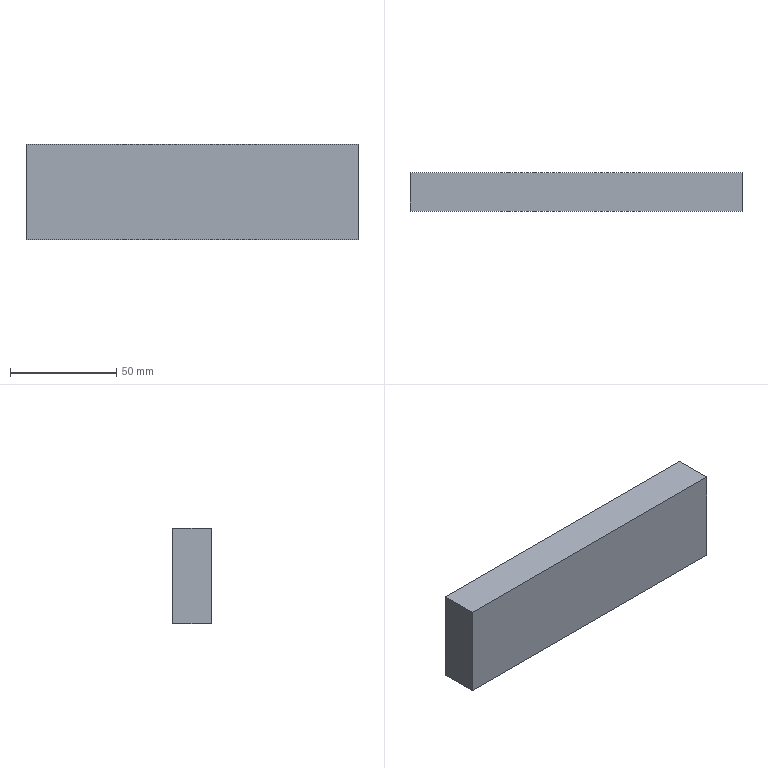NC program | NX | posted with a generic post | part box 156 x 18 x 45 mm
Lines 1 to 1294 of 3545:
N10 G17 G21 G94 G90
(PLANAR_MILL , TOOL : D16C)
N12 T01 M6
N14 G54
N16 G17 G0 G90 X-90. Y0. S2300 M3
N18 G43 Z20. H1
N20 Z3.
N22 G94 G1 Z0. F800.
N24 X-74.
N26 X74.
N28 X90.
N30 Z3.
N32 G0 Z20.
(ADAPTIVE_MILLING , TOOL : D16C)
N34 X93.024 Y6.776 S3500
N36 Z-38.
N38 G1 X92.875 Y6.789 Z-38.937 F1500.
N40 X92.725 Y6.801 Z-39.308
N42 X92.576 Y6.813 Z-39.58
N44 X92.426 Y6.826 Z-39.8
N46 X92.277 Y6.838 Z-39.984
N48 X92.127 Y6.85 Z-40.142
N50 X91.978 Y6.863 Z-40.28
N52 X91.828 Y6.875 Z-40.4
N54 X91.679 Y6.887 Z-40.505
N56 X91.529 Y6.9 Z-40.598
N58 X91.38 Y6.912 Z-40.679
N60 X91.231 Y6.924 Z-40.75
N62 X91.081 Y6.937 Z-40.81
N64 X90.932 Y6.949 Z-40.862
N66 X90.782 Y6.961 Z-40.905
N68 X90.633 Y6.974 Z-40.939
N70 X90.483 Y6.986 Z-40.966
N72 X90.334 Y6.998 Z-40.985
N74 X90.184 Y7.011 Z-40.996
N76 X90.035 Y7.023 Z-41.
N78 X87.714 Y7.215
N80 G3 X86.001 Y5.942 R1.616
N82 X85.745 Y2.219 R24.863
N84 X85.69 Y-7.255 R731.999
N86 G2 X82.243 Y-13.665 R8.873
N88 X76.479 Y-16.159 R12.982
N90 X70.319 Y-16.657 R37.349
N92 X60.044 Y-16.7 R710.459
N94 G1 X-75.926
N96 G2 X-82.503 Y-13.438 R8.777
N98 X-85.116 Y-7.695 R12.719
N100 X-85.653 Y-1.502 R35.427
N102 X-85.678 Y7.423 R259.053
N104 X-82.107 Y13.763 R8.94
N106 X-76.314 Y16.188 R13.167
N108 X-70.377 Y16.655 R37.978
N110 X-60.252 Y16.7 R702.362
N112 G1 X76.02 Y16.698
N114 G2 X82.504 Y13.429 R8.805
N116 X85.03 Y7.644 R11.914
N118 X85.396 Y1.962 R36.217
N120 X85.378 Y-5.456 R267.86
N122 X80.394 Y-13.694 R10.594
N124 X74.115 Y-15.922 R15.915
N126 X67.459 Y-16.36 R49.943
N128 X57.034 Y-16.399 R727.387
N130 G1 X-73.776
N132 G2 X-82.645 Y-11.469 R10.563
N134 X-84.903 Y-5.239 R15.759
N136 X-85.356 Y1.303 R47.673
N138 X-85.348 Y5.689 R58.15
N140 X-80.369 Y13.704 R10.603
N142 X-74.26 Y15.898 R15.81
N144 X-67.344 Y16.362 R49.309
N146 X-58.119 Y16.399 R683.552
N148 G1 X73.914 Y16.397
N150 G2 X82.791 Y11.121 R10.428
N152 X84.753 Y4.979 R15.923
N154 X85.085 Y-1.983 R59.735
N156 X84.675 Y-6.373 R15.473
N158 X78.65 Y-13.752 R11.862
N160 X72.18 Y-15.676 R18.719
N162 X65.032 Y-16.065 R63.475
N164 G1 X54.757 Y-16.099
N166 X-72.087 Y-16.097
N168 G2 X-82.601 Y-9.926 R11.776
N170 X-84.63 Y-3.518 R18.113
N172 X-85.016 Y4.076 R47.717
N174 X-79.074 Y13.505 R11.652
N176 X-72.582 Y15.618 R17.858
N178 X-65.101 Y16.064 R59.034
N180 G1 X-54.751 Y16.099
N182 X71.888
N184 G2 X79.569 Y13.489 R11.642
N186 X83.651 Y7.131 R13.214
N188 X84.661 Y0.626 R26.639
N190 X84.592 Y-3.941 R24.232
N192 X82.297 Y-9.622 R12.908
N194 G1 X81.593 Y-10.791
N196 G2 X79.789 Y-12.594 R9.495
N198 X76.093 Y-14.321 R13.778
N200 X68.797 Y-15.587 R29.634
N202 X59.125 Y-15.792 R167.5
N204 G1 X52.825 Y-15.799
N206 X-71.108 Y-15.792
N208 G2 X-78.673 Y-13.273 R13.032
N210 X-80.764 Y-11.762 R9.397
N212 X-82.832 Y-8.434 R9.597
N214 X-84.494 Y-0.994 R25.738
N216 X-84.56 Y3.722 R23.424
N218 X-82.359 Y9.479 R12.307
N220 X-81.593 Y10.791 R11.314
N222 X-79.789 Y12.594 R9.495
N224 X-76.126 Y14.308 R13.699
N226 X-68.905 Y15.579 R29.459
N228 X-59.459 Y15.791 R157.993
N230 G1 X-52.859 Y15.798
N232 X71.104 Y15.792
N234 G2 X78.874 Y13.025 R12.62
N236 G1 X79.791 Y12.463
N238 G2 X81.594 Y10.659 R9.495
N240 X82.435 Y9.194 R10.523
N242 X84.216 Y1.4 R25.74
N244 X83.999 Y-4.16 R18.18
N246 X83.097 Y-6.98 R20.614
N248 G1 X83.059 Y-7.164
N250 G3 X83.597 Y-8.552 R1.601
N252 X84.161 Y-8.878 Z-40.979 R1.942
N254 G1 X86.488 Y-9.882 Z-40.9
N256 X87.519 Y-10.327 F15000.
N258 G2 X86.647 Y-13.378 R1.6
N260 G1 X85.769 Y-13.25
N262 X84.762 Y-13.23
N264 X81.573 Y-13.177 Z-41. F1500.
N266 X79.337 Y-13.141
N268 G3 X78.699 Y-13.262 R1.629
N270 G1 X77.517 Y-13.751
N272 G2 X65.466 Y-15.396 R50.543
N274 X51.291 Y-15.498 R552.582
N276 G1 X-70.945 Y-15.497
N278 G2 X-76.206 Y-14.066 R17.016
N280 G1 X-77.52 Y-13.751
N282 X-78.697 Y-13.263
N284 G3 X-80.899 Y-14.551 R1.6
N286 X-80.499 Y-15.822 Z-40.957 R1.683
N288 G1 X-79.408 Y-17.277 Z-40.9
N290 X-78.351 Y-18.687 F15000.
N292 G3 X-77.072 Y-19.328 R1.601
N294 G1 X73.134 Y-19.488
N296 G3 X74.042 Y-19.206 R1.606
N298 G1 X75.642 Y-18.107
N300 X76.516 Y-17.511 Z-40.933 F1500.
N302 X77.382 Y-16.903 Z-40.966
N304 G3 X77.954 Y-16.021 Z-41. R1.6
N306 X76.274 Y-14.05 R1.6
N308 X71.939 Y-14.58 R95.722
N310 G2 X61.46 Y-15.159 R95.011
N312 X50.51 Y-15.198 R758.856
N314 G1 X-70.92 Y-15.197
N316 G2 X-74.563 Y-14.26 R24.752
N318 G1 X-75.033 Y-14.147
N320 G2 X-76.458 Y-14.006 R10.128
N322 G3 X-78.339 Y-16.099 R1.6
N324 X-77.575 Y-16.987 Z-40.963 R1.702
N326 G1 X-75.904 Y-18.072 Z-40.9
N328 X-74.189 Y-19.185 F15000.
N330 G3 X-73.319 Y-19.443 R1.608
N332 G1 X72.573 Y-19.532
N334 G3 X73.481 Y-19.25 R1.606
N336 G1 X75.095 Y-18.141
N338 X76.812 Y-16.956 Z-40.965 F1500.
N340 G3 X77.398 Y-16.048 Z-41. R1.601
N342 X75.713 Y-14.094 R1.6
N344 G2 X73.463 Y-14.201 R70.607
N346 X58.022 Y-14.88 R160.391
N348 G1 X48.722 Y-14.897
N350 X-68.72 Y-14.896
N352 G2 X-73.459 Y-14.172 R28.882
N354 G3 X-75.038 Y-14.147 R19.275
N356 X-76.744 Y-15.99 R1.6
N358 X-76.07 Y-17.061 Z-40.959 R1.617
N360 G1 X-74.513 Y-18.13 Z-40.9
N362 X-72.804 Y-19.304 F15000.
N364 G3 X-71.898 Y-19.585 R1.606
N366 G1 X71.372 Y-19.588
N368 G3 X72.301 Y-19.291 R1.605
N370 G1 X73.908 Y-18.146
N372 X74.713 Y-17.574 Z-40.931 F1500.
N374 X75.513 Y-16.994 Z-40.962
N376 G3 X76.097 Y-15.965 Z-41. R1.6
N378 X74.512 Y-14.15 R1.6
N380 X67.386 Y-14.354 R97.044
N382 G2 X52.801 Y-14.594 R328.555
N384 G1 X47.626 Y-14.597
N386 X-68.72 Y-14.596
N388 G2 X-71.854 Y-14.15 R102.479
N390 G1 X-73.692
N392 G3 X-75.281 Y-15.935 R1.6
N394 X-74.622 Y-17.051 Z-40.958 R1.617
N396 G1 X-73.114 Y-18.13 Z-40.9
N398 X-71.494 Y-19.289 F15000.
N400 G3 X-70.552 Y-19.588 R1.605
N402 G1 X67.597 Y-18.59
N404 X67.807 Y-18.573
N406 X68.015 Y-18.531
N408 X69.418 Y-18.14
N410 X72.49 Y-17.284 Z-41. F1500.
N412 G3 X72.037 Y-14.15 R1.6
N414 X58.515 Y-14.265 R663.31
N416 G1 X47.34 Y-14.297
N418 X-66.61 Y-14.293
N420 G2 X-68.97 Y-14.15 R55.681
N422 G1 X-71.857
N424 G3 X-72.343 Y-17.274 R1.6
N426 G1 X-69.272 Y-18.133 Z-40.9
N428 X-68.49 Y-18.354 F15000.
N430 X-67.706 Y-18.564
N432 X-67.417 Y-18.59
N434 X61.934
N436 X62.151 Y-18.573
N438 X62.365 Y-18.531
N440 X63.761 Y-18.141
N442 X66.833 Y-17.283 Z-41. F1500.
N444 G3 X66.374 Y-14.15 R1.6
N446 G1 X-75.001
N448 G2 X-77.52 Y-13.751 R9.498
N450 X-79.791 Y-12.593 R9.495
N452 X-81.594 Y-10.789 R9.495
N454 X-82.751 Y-8.517 R9.495
N456 X-84.2 Y0.015 R46.979
N458 X-83.114 Y6.806 R15.168
N460 G1 X-83.069 Y7.026
N462 G3 X-84.767 Y8.747 R1.6
N464 X-85.905 Y8.161 Z-40.959 R1.617
N466 G1 X-87.087 Y6.709 Z-40.9
N468 X-88.925 Y4.452 F15000.
N470 G3 X-89.284 Y3.438 R1.603
N472 G1 X-89.264 Y-3.686
N474 G3 X-88.906 Y-4.69 R1.604
N476 G1 X-87.084 Y-6.933
N478 X-85.825 Y-8.476 Z-40.962 F1500.
N480 G3 X-84.777 Y-8.994 Z-41. R1.6
N482 X-83.05 Y-7.274 R1.6
N484 X-83.574 Y-2.989 R93.564
N486 G2 X-83.595 Y2.99 R20.7
N488 G1 X-83.151 Y5.291
N490 G2 X-83.049 Y7.276 R15.825
N492 G1 X-82.751 Y8.52
N494 X-82.32 Y9.559
N496 G3 X-84.889 Y11.342 R1.6
N498 G1 X-85.092 Y11.113 Z-40.99
N500 X-85.272 Y10.865 Z-40.981
N502 X-86.783 Y8.779 Z-40.9
N504 X-88.236 Y6.774 F15000.
N506 G3 X-88.535 Y5.971 R1.61
N508 G1 X-89.309 Y-3.125
N510 G3 X-88.936 Y-4.294 R1.602
N512 G1 X-87.126 Y-6.434
N514 X-86.49 Y-7.19 Z-40.931 F1500.
N516 X-85.846 Y-7.939 Z-40.962
N518 G3 X-84.773 Y-8.436 Z-41. R1.6
N520 X-83.094 Y-6.713 R1.6
N522 G2 X-83.202 Y-4.439 R74.089
N524 X-83.395 Y0.423 R39.504
N526 X-83.15 Y2.998 R43.005
N528 G1 Y5.332
N530 G3 X-85.913 Y6.431 R1.6
N532 X-86.306 Y5.737 Z-40.975 R1.812
N534 G1 X-87.133 Y3.499 Z-40.9
N536 X-88.125 Y0.812 F15000.
N538 G3 X-88.224 Y0.258 R1.667
N540 G1 X-88.226 Y-0.184
N542 X-88.213 Y-0.626
N544 X-88.178 Y-0.811
N546 X-88.125 Y-0.992
N548 X-87.141 Y-3.655
N550 X-86.251 Y-6.066 Z-40.981 F1500.
N552 G3 X-85.931 Y-6.592 Z-41. R1.636
N554 X-83.15 Y-5.512 R1.6
N556 G1 Y6.001
N558 G2 X-82.751 Y8.52 R9.498
N560 X-81.593 Y10.791 R9.495
N562 X-79.789 Y12.594 R9.495
N564 X-77.517 Y13.751 R9.495
N566 X-65.692 Y15.388 R50.154
N568 X-51.293 Y15.498 R516.951
N570 G1 X70.907 Y15.497
N572 G2 X76.456 Y13.882 R16.043
N574 X78.893 Y13.013 R8.415
N576 G3 X81.329 Y14.401 R1.6
N578 X80.886 Y15.493 Z-40.962 R1.701
N580 G1 X79.651 Y17.047 Z-40.9
N582 X78.516 Y18.474 F15000.
N584 G3 X77.268 Y19.079 R1.601
N586 G1 X-73.134 Y19.488
N588 G3 X-74.045 Y19.206 R1.606
N590 G1 X-75.643 Y18.107
N592 X-76.517 Y17.511 Z-40.933 F1500.
N594 X-77.383 Y16.903 Z-40.966
N596 G3 X-77.955 Y16.019 Z-41. R1.6
N598 X-76.274 Y14.05 R1.6
N600 X-71.912 Y14.583 R96.343
N602 G2 X-61.433 Y15.159 R95.363
N604 X-50.334 Y15.198 R764.363
N606 G1 X70.891 Y15.197
N608 G2 X74.679 Y14.163 R21.713
N610 G3 X75.293 Y13.997 R10.655
N612 G2 X76.531 Y13.858 R6.686
N614 G3 X78.403 Y15.976 R1.6
N616 X77.646 Y16.84 Z-40.963 R1.707
N618 G1 X75.955 Y17.938 Z-40.9
N620 X74.26 Y19.038 F15000.
N622 G3 X73.392 Y19.296 R1.608
N624 G1 X-72.573 Y19.532
N626 G3 X-73.482 Y19.25 R1.606
N628 G1 X-75.096 Y18.141
N630 X-76.812 Y16.956 Z-40.965 F1500.
N632 G3 X-77.398 Y16.047 Z-41. R1.601
N634 X-75.713 Y14.094 R1.6
N636 G2 X-73.44 Y14.202 R73.267
N638 X-57.996 Y14.88 R160.551
N640 G1 X-48.696 Y14.897
N642 X70.328 Y14.898
N644 G2 X72.74 Y14.355 R16.77
N646 G3 X74.167 Y14.02 R11.704
N648 G2 X75.3 Y13.996 R29.277
N650 G3 X77. Y15.876 R1.6
N652 X76.209 Y16.994 Z-40.956 R1.677
N654 G1 X74.744 Y18. Z-40.9
N656 X73.064 Y19.153 F15000.
N658 G3 X72.16 Y19.434 R1.606
N660 G1 X-71.372 Y19.588
N662 G3 X-72.303 Y19.291 R1.605
N664 G1 X-73.908 Y18.146
N666 X-74.714 Y17.574 Z-40.931 F1500.
N668 X-75.514 Y16.994 Z-40.962
N670 G3 X-76.097 Y15.964 Z-41. R1.6
N672 X-74.512 Y14.15 R1.6
N674 X-67.173 Y14.364 R103.503
N676 G2 X-52.851 Y14.593 R332.279
N678 G1 X-47.601 Y14.597
N680 X69.293
N682 G2 X72.647 Y14.021 R67.717
N684 G1 X74.184 Y14.02
N686 G3 X75.773 Y15.805 R1.6
N688 X75.115 Y16.921 Z-40.958 R1.617
N690 G1 X73.606 Y18. Z-40.9
N692 X71.985 Y19.159 F15000.
N694 G3 X71.045 Y19.458 R1.605
N696 G1 X-67.634 Y18.59
N698 X-67.846 Y18.573
N700 X-68.054 Y18.531
N702 X-69.457 Y18.14
N704 X-72.529 Y17.284 Z-41. F1500.
N706 G3 X-72.074 Y14.15 R1.6
N708 X-58.452 Y14.266 R673.335
N710 G1 X-47.127 Y14.297
N712 X68.408 Y14.296
N714 X70.609 Y14.02
N716 X72.709
N718 G3 X74.298 Y15.805 R1.6
N720 X73.64 Y16.921 Z-40.958 R1.617
N722 G1 X72.131 Y18. Z-40.9
N724 X70.511 Y19.159 F15000.
N726 G3 X69.569 Y19.458 R1.605
N728 G1 X-61.934 Y18.59
N730 X-62.146 Y18.573
N732 X-62.353 Y18.531
N734 X-63.756 Y18.14
N736 X-66.829 Y17.284 Z-41. F1500.
N738 G3 X-66.374 Y14.15 R1.6
N740 G1 X54.5
N742 G3 X60.001 Y14.02 R82.862
N744 G1 X70.613
N746 G3 X71.704 Y16.79 R1.6
N748 X71.024 Y17.174 Z-40.975 R1.783
N750 G1 X68.769 Y18.003 Z-40.9
N752 X66.067 Y18.996 F15000.
N754 G3 X65.539 Y19.094 R1.682
N756 G1 X60.436 Y19.171
N758 G3 X59.844 Y19.068 R1.64
N760 G1 X56.792 Y17.91
N762 X55.796 Y17.536 Z-40.933 F1500.
N764 X54.804 Y17.151 Z-40.967
N766 G3 X54.044 Y16.439 Z-41. R1.6
N768 X55.361 Y14.097 R1.6
N770 X58.272 Y13.823 R18.352
N772 G1 X58.383 Y13.839
N774 G3 X58.195 Y17.312 R1.76
N776 G1 X56.437 Y17.488
N778 G3 X55.94 Y14.006 R1.76
N780 X57.744 Y13.716 R12.424
N782 X58.7 Y13.916 R6.013
N784 G1 X59.896 Y14.012
N786 G3 X59.639 Y17.522 R1.76
N788 G1 X56.894 Y17.34
N790 G3 X56.48 Y13.906 R1.76
N792 X57.713 Y13.684 R2.819
N794 G1 X58.018 Y13.748
N796 G3 X57.273 Y17.187 R1.76
N798 X55.768 Y15.843 R1.792
N800 X56.945 Y13.759 R1.76
N802 X58.229 Y13.796 R2.153
N804 G1 X58.7 Y13.916
N806 X60.001 Y14.02
N808 X75.001
N810 G2 X77.52 Y13.621 R9.498
N812 X79.791 Y12.463 R9.495
N814 X81.594 Y10.659 R9.495
N816 X82.751 Y8.387 R9.495
N818 X83.606 Y3.684 R39.624
N820 X83.803 Y-2.072 R23.31
N822 X83.158 Y-5.447 R35.619
N824 X83.049 Y-7.276 R22.868
N826 X82.277 Y-9.663 R9.423
N828 G3 X84.875 Y-11.418 R1.6
N830 G1 X85.062 Y-11.199 Z-40.991
N832 X85.231 Y-10.966 Z-40.982
N834 X86.766 Y-8.851 Z-40.9
N836 X88.192 Y-6.887 F15000.
N838 G3 X88.492 Y-6.075 R1.609
N840 G1 X89.264 Y3.556
N842 G3 X88.893 Y4.715 R1.602
N844 G1 X87.083 Y6.861
N846 X86.447 Y7.618 Z-40.931 F1500.
N848 X85.804 Y8.369 Z-40.962
N850 G3 X84.731 Y8.867 Z-41. R1.6
N852 X83.05 Y7.144 R1.6
N854 G2 X83.492 Y1.524 R292.083
N856 X83.15 Y-3.478 R26.196
N858 G1 Y-5.578
N860 G3 X84.75 Y-7.178 R1.6
N862 X85.975 Y-6.607 Z-40.956 R1.612
N864 G1 X87.129 Y-5.233 Z-40.9
N866 X88.99 Y-3.019 F15000.
N868 G3 X89.365 Y-1.989 R1.603
N870 G1 Y2.281
N872 G3 X88.99 Y3.311 R1.603
N874 G1 X87.148 Y5.503
N876 X86.533 Y6.24 Z-40.93 F1500.
N878 X85.908 Y6.969 Z-40.96
N880 G3 X84.779 Y7.469 Z-41. R1.599
N882 X83.15 Y5.869 R1.6
N884 G2 X83.15 Y-3.503 R737.034
N886 G3 X84.75 Y-5.103 R1.6
N888 X85.975 Y-4.532 Z-40.956 R1.612
N890 G1 X87.129 Y-3.159 Z-40.9
N892 X88.99 Y-0.944 F15000.
N894 G3 X89.365 Y0.085 R1.603
N896 X89.322 Y0.738 R2.708
N898 X88.99 Y1.398 R1.617
N900 G1 X87.148 Y3.591
N902 X86.533 Y4.328 Z-40.93 F1500.
N904 X85.908 Y5.057 Z-40.96
N906 G3 X84.779 Y5.557 Z-41. R1.599
N908 X83.15 Y3.957 R1.6
N910 G1 Y0.469
N912 G3 X84.543 Y-1.131 R1.616
N914 G1 X87.137 Y-1.492
N916 X87.285 Y-1.513 Z-40.996
N918 X87.434 Y-1.534 Z-40.985
N920 X87.582 Y-1.554 Z-40.966
N922 X87.731 Y-1.575 Z-40.939
N924 X87.88 Y-1.596 Z-40.905
N926 X88.028 Y-1.617 Z-40.862
N928 X88.177 Y-1.637 Z-40.81
N930 X88.325 Y-1.658 Z-40.75
N932 X88.474 Y-1.679 Z-40.679
N934 X88.622 Y-1.699 Z-40.598
N936 X88.771 Y-1.72 Z-40.505
N938 X88.92 Y-1.741 Z-40.4
N940 X89.068 Y-1.761 Z-40.28
N942 X89.217 Y-1.782 Z-40.142
N944 X89.365 Y-1.803 Z-39.984
N946 X89.514 Y-1.823 Z-39.8
N948 X89.662 Y-1.844 Z-39.58
N950 X89.811 Y-1.865 Z-39.308
N952 X89.959 Y-1.886 Z-38.937
N954 X90.108 Y-1.906 Z-38.
N956 G0 Z20.
N958 M5
(PLANAR_MILL_1 , TOOL : D14J)
N960 T02 M6
N962 G54
N964 G17 G0 G90 X55.513 Y15.492 S3000 M3
N966 G43 Z20. H2
N968 Z-39.
N970 G94 G1 Z-41. F600.
N972 G41 X55.426 Y15. D2
N974 G3 X57.426 Y13. R2.
N976 G1 X75.
N978 G2 X82. Y6. R7.
N980 G1 Y-6.
N982 G2 X75. Y-13. R7.
N984 G1 X-75.
N986 G2 X-82. Y-6. R7.
N988 G1 Y6.
N990 G2 X-75. Y13. R7.
N992 G1 X57.426
N994 G3 X59.426 Y15. R2.
N996 G40
N998 G1 X59.339 Y15.492
N1000 X55.513
N1002 G41 X55.426 Y15.
N1004 G3 X57.426 Y13. R2.
N1006 G1 X75.
N1008 G2 X82. Y6. R7.
N1010 G1 Y-6.
N1012 G2 X75. Y-13. R7.
N1014 G1 X-75.
N1016 G2 X-82. Y-6. R7.
N1018 G1 Y6.
N1020 G2 X-75. Y13. R7.
N1022 G1 X57.426
N1024 G3 X59.426 Y15. R2.
N1026 G40
N1028 G1 X59.339 Y15.492
N1030 Z-39.
N1032 G0 Z20.
(PLANAR_MILL_1_COPY_1 , TOOL : D14J)
N1034 X57.087 Y15.362
N1036 Z-39.
N1038 G1 Z-41.
N1040 G41 X57. Y14.87
N1042 G3 X59. Y12.87 R2.
N1044 G1 X75.5
N1046 G3 X77.5 Y14.87 R2.
N1048 G40
N1050 G1 X77.413 Y15.362
N1052 Z-39.
N1054 G0 Z20.
N1056 X57.087
N1058 Z-39.
N1060 G1 Z-41.
N1062 G41 X57. Y14.87
N1064 G3 X59. Y12.87 R2.
N1066 G1 X75.5
N1068 G3 X77.5 Y14.87 R2.
N1070 G40
N1072 G1 X77.413 Y15.362
N1074 Z-39.
N1076 G0 Z20.
N1078 M5
(PLANAR_MILL_2 , TOOL : D4C)
N1080 T03 M6
N1082 G54
N1084 G17 G0 G90 X-5.194 Y1.15 S3500 M3
N1086 G43 Z20. H3
N1088 Z0.5
N1090 G94 G1 X-69.264 Z0.444 F1500.
N1092 X-69.834 Y0.834
N1094 X-70.15 Y0.264 Z0.443
N1096 Y-0.264 Z0.442
N1098 X-69.834 Y-0.834
N1100 X-69.264 Y-1.15 Z0.441
N1102 X46.264 Z0.341
N1104 G3 X46.958 Y0.689 R1.222
N1106 G1 X46.653 Y0.983 Z0.338
N1108 X46.264 Y1.15
N1110 X-69.264 Z0.237
N1112 X-69.834 Y0.834 Z0.236
N1114 X-70.15 Y0.264
N1116 Y-0.264 Z0.235
N1118 X-69.834 Y-0.834
N1120 X-69.264 Y-1.15 Z0.234
N1122 X46.264 Z0.133
N1124 G3 X46.958 Y0.689 R1.222
N1126 G1 X46.653 Y0.983 Z0.131
N1128 X46.264 Y1.15
N1130 X-69.264 Z0.03
N1132 X-69.834 Y0.834 Z0.029
N1134 X-70.15 Y0.264
N1136 Y-0.264 Z0.028
N1138 X-69.834 Y-0.834
N1140 X-69.264 Y-1.15 Z0.027
N1142 X46.264 Z-0.074
N1144 G3 X46.958 Y0.689 R1.222
N1146 G1 X46.653 Y0.983 Z-0.076
N1148 X46.264 Y1.15
N1150 X-69.264 Z-0.177
N1152 X-69.834 Y0.834 Z-0.178
N1154 X-70.15 Y0.264
N1156 Y-0.264 Z-0.179
N1158 X-69.834 Y-0.834
N1160 X-69.264 Y-1.15 Z-0.18
N1162 X46.264 Z-0.281
N1164 G3 X46.958 Y0.689 R1.222
N1166 G1 X46.653 Y0.983 Z-0.283
N1168 X46.264 Y1.15 Z-0.284
N1170 X-69.264 Z-0.384
N1172 X-69.834 Y0.834 Z-0.385
N1174 X-70.15 Y0.264
N1176 Y-0.264 Z-0.386
N1178 X-69.834 Y-0.834 Z-0.387
N1180 X-69.264 Y-1.15
N1182 X46.264 Z-0.488
N1184 G3 X46.958 Y0.689 R1.222
N1186 G1 X46.653 Y0.983 Z-0.49
N1188 X46.264 Y1.15 Z-0.491
N1190 X-69.264 Z-0.591
N1192 X-69.834 Y0.834 Z-0.592
N1194 X-70.15 Y0.264 Z-0.593
N1196 Y-0.264
N1198 X-69.834 Y-0.834 Z-0.594
N1200 X-69.264 Y-1.15
N1202 X46.264 Z-0.695
N1204 G3 X46.958 Y0.689 R1.222
N1206 G1 X46.653 Y0.983 Z-0.697
N1208 X46.264 Y1.15 Z-0.698
N1210 X-69.264 Z-0.799
N1212 X-69.834 Y0.834
N1214 X-70.15 Y0.264 Z-0.8
N1216 Y-0.264
N1218 X-69.834 Y-0.834 Z-0.801
N1220 X-69.264 Y-1.15
N1222 X46.264 Z-0.902
N1224 G3 X46.958 Y0.689 R1.222
N1226 G1 X46.653 Y0.983 Z-0.904
N1228 X46.264 Y1.15 Z-0.905
N1230 X-69.264 Z-1.006
N1232 X-69.834 Y0.834
N1234 X-70.15 Y0.264 Z-1.007
N1236 Y-0.264
N1238 X-69.834 Y-0.834 Z-1.008
N1240 X-69.264 Y-1.15
N1242 X46.264 Z-1.109
N1244 G3 X46.958 Y0.689 R1.222
N1246 G1 X46.653 Y0.983 Z-1.112
N1248 X46.264 Y1.15
N1250 X-69.264 Z-1.213
N1252 X-69.834 Y0.834
N1254 X-70.15 Y0.264 Z-1.214
N1256 Y-0.264
N1258 X-69.834 Y-0.834 Z-1.215
N1260 X-69.264 Y-1.15 Z-1.216
N1262 X46.264 Z-1.316
N1264 G3 X46.958 Y0.689 R1.222
N1266 G1 X46.653 Y0.983 Z-1.319
N1268 X46.264 Y1.15
N1270 X-69.264 Z-1.42
N1272 X-69.834 Y0.834
N1274 X-70.15 Y0.264 Z-1.421
N1276 Y-0.264
N1278 X-69.834 Y-0.834 Z-1.422
N1280 X-69.264 Y-1.15 Z-1.423
N1282 X46.264 Z-1.523
N1284 G3 X46.958 Y0.689 R1.222
N1286 G1 X46.653 Y0.983 Z-1.526
N1288 X46.264 Y1.15
N1290 X-69.264 Z-1.627
N1292 X-69.834 Y0.834 Z-1.628
N1294 X-70.15 Y0.264
N1296 Y-0.264 Z-1.629
N1298 X-69.834 Y-0.834
N1300 X-69.264 Y-1.15 Z-1.63
N1302 X46.264 Z-1.731
N1304 G3 X46.958 Y0.689 R1.222
N1306 G1 X46.653 Y0.983 Z-1.733
N1308 X46.264 Y1.15
N1310 X-69.264 Z-1.834
N1312 X-69.834 Y0.834 Z-1.835
N1314 X-70.15 Y0.264
N1316 Y-0.264 Z-1.836
N1318 X-69.834 Y-0.834
N1320 X-69.264 Y-1.15 Z-1.837
N1322 X46.264 Z-1.938
N1324 G3 X46.958 Y0.689 R1.222
N1326 G1 X46.653 Y0.983 Z-1.94
N1328 X46.264 Y1.15
N1330 X-69.264 Z-2.041
N1332 X-69.834 Y0.834 Z-2.042
N1334 X-70.15 Y0.264
N1336 Y-0.264 Z-2.043
N1338 X-69.834 Y-0.834
N1340 X-69.264 Y-1.15 Z-2.044
N1342 X46.264 Z-2.145
N1344 G3 X46.958 Y0.689 R1.222
N1346 G1 X46.653 Y0.983 Z-2.147
N1348 X46.264 Y1.15 Z-2.148
N1350 X-69.264 Z-2.248
N1352 X-69.834 Y0.834 Z-2.249
N1354 X-70.15 Y0.264
N1356 Y-0.264 Z-2.25
N1358 X-69.834 Y-0.834
N1360 X-69.264 Y-1.15 Z-2.251
N1362 X46.264 Z-2.352
N1364 G3 X46.958 Y0.689 R1.222
N1366 G1 X46.653 Y0.983 Z-2.354
N1368 X46.264 Y1.15 Z-2.355
N1370 X-69.264 Z-2.455
N1372 X-69.834 Y0.834 Z-2.456
N1374 X-70.15 Y0.264 Z-2.457
N1376 Y-0.264
N1378 X-69.834 Y-0.834 Z-2.458
N1380 X-69.264 Y-1.15
N1382 X46.264 Z-2.559
N1384 G3 X46.958 Y0.689 R1.222
N1386 G1 X46.653 Y0.983 Z-2.561
N1388 X46.264 Y1.15 Z-2.562
N1390 X-69.264 Z-2.663
N1392 X-69.834 Y0.834
N1394 X-70.15 Y0.264 Z-2.664
N1396 Y-0.264
N1398 X-69.834 Y-0.834 Z-2.665
N1400 X-69.264 Y-1.15
N1402 X46.264 Z-2.766
N1404 G3 X46.958 Y0.689 R1.222
N1406 G1 X46.653 Y0.983 Z-2.768
N1408 X46.264 Y1.15 Z-2.769
N1410 X-69.264 Z-2.87
N1412 X-69.834 Y0.834
N1414 X-70.15 Y0.264 Z-2.871
N1416 Y-0.264
N1418 X-69.834 Y-0.834 Z-2.872
N1420 X-69.264 Y-1.15
N1422 X46.264 Z-2.973
N1424 G3 X46.958 Y0.689 R1.222
N1426 G1 X46.653 Y0.983 Z-2.976
N1428 X46.264 Y1.15
N1430 X-69.264 Z-3.077
N1432 X-69.834 Y0.834
N1434 X-70.15 Y0.264 Z-3.078
N1436 Y-0.264
N1438 X-69.834 Y-0.834 Z-3.079
N1440 X-69.264 Y-1.15
N1442 X46.264 Z-3.18
N1444 G3 X46.958 Y0.689 R1.222
N1446 G1 X46.653 Y0.983 Z-3.183
N1448 X46.264 Y1.15
N1450 X-69.264 Z-3.284
N1452 X-69.834 Y0.834
N1454 X-70.15 Y0.264 Z-3.285
N1456 Y-0.264
N1458 X-69.834 Y-0.834 Z-3.286
N1460 X-69.264 Y-1.15 Z-3.287
N1462 X46.264 Z-3.387
N1464 G3 X46.958 Y0.689 R1.222
N1466 G1 X46.653 Y0.983 Z-3.39
N1468 X46.264 Y1.15
N1470 X-69.264 Z-3.491
N1472 X-69.834 Y0.834 Z-3.492
N1474 X-70.15 Y0.264
N1476 Y-0.264 Z-3.493
N1478 X-69.834 Y-0.834
N1480 X-69.264 Y-1.15 Z-3.494
N1482 X46.264 Z-3.595
N1484 G3 X46.958 Y0.689 R1.222
N1486 G1 X46.653 Y0.983 Z-3.597
N1488 X46.264 Y1.15
N1490 X-69.264 Z-3.698
N1492 X-69.834 Y0.834 Z-3.699
N1494 X-70.15 Y0.264
N1496 Y-0.264 Z-3.7
N1498 X-69.834 Y-0.834
N1500 X-69.264 Y-1.15 Z-3.701
N1502 X46.264 Z-3.802
N1504 G3 X46.958 Y0.689 R1.222
N1506 G1 X46.653 Y0.983 Z-3.804
N1508 X46.264 Y1.15
N1510 X-69.264 Z-3.905
N1512 X-69.834 Y0.834 Z-3.906
N1514 X-70.15 Y0.264
N1516 Y-0.264 Z-3.907
N1518 X-69.834 Y-0.834
N1520 X-69.264 Y-1.15 Z-3.908
N1522 X46.264 Z-4.009
N1524 G3 X46.958 Y0.689 R1.222
N1526 G1 X46.653 Y0.983 Z-4.011
N1528 X46.264 Y1.15
N1530 X-69.264 Z-4.112
N1532 X-69.834 Y0.834 Z-4.113
N1534 X-70.15 Y0.264
N1536 Y-0.264 Z-4.114
N1538 X-69.834 Y-0.834
N1540 X-69.264 Y-1.15 Z-4.115
N1542 X46.264 Z-4.216
N1544 G3 X46.958 Y0.689 R1.222
N1546 G1 X46.653 Y0.983 Z-4.218
N1548 X46.264 Y1.15 Z-4.219
N1550 X-69.264 Z-4.319
N1552 X-69.834 Y0.834 Z-4.32
N1554 X-70.15 Y0.264 Z-4.321
N1556 Y-0.264
N1558 X-69.834 Y-0.834 Z-4.322
N1560 X-69.264 Y-1.15
N1562 X46.264 Z-4.423
N1564 G3 X46.958 Y0.689 R1.222
N1566 G1 X46.653 Y0.983 Z-4.425
N1568 X46.264 Y1.15 Z-4.426
N1570 X-69.264 Z-4.527
N1572 X-69.834 Y0.834
N1574 X-70.15 Y0.264 Z-4.528
N1576 Y-0.264
N1578 X-69.834 Y-0.834 Z-4.529
N1580 X-69.264 Y-1.15
N1582 X46.264 Z-4.63
N1584 G3 X46.958 Y0.689 R1.222
N1586 G1 X46.653 Y0.983 Z-4.632
N1588 X46.264 Y1.15 Z-4.633
N1590 X-69.264 Z-4.734
N1592 X-69.834 Y0.834
N1594 X-70.15 Y0.264 Z-4.735
N1596 Y-0.264
N1598 X-69.834 Y-0.834 Z-4.736
N1600 X-69.264 Y-1.15
N1602 X46.264 Z-4.837
N1604 G3 X46.958 Y0.689 R1.222
N1606 G1 X46.653 Y0.983 Z-4.84
N1608 X46.264 Y1.15
N1610 X-69.264 Z-4.941
N1612 X-69.834 Y0.834
N1614 X-70.15 Y0.264 Z-4.942
N1616 Y-0.264
N1618 X-69.834 Y-0.834 Z-4.943
N1620 X-69.264 Y-1.15
N1622 X46.264 Z-5.044
N1624 G3 X46.958 Y0.689 R1.222
N1626 G1 X46.653 Y0.983 Z-5.047
N1628 X46.264 Y1.15
N1630 X-69.264 Z-5.148
N1632 X-69.834 Y0.834
N1634 X-70.15 Y0.264 Z-5.149
N1636 Y-0.264
N1638 X-69.834 Y-0.834 Z-5.15
N1640 X-69.264 Y-1.15 Z-5.151
N1642 X46.264 Z-5.251
N1644 G3 X46.958 Y0.689 R1.222
N1646 G1 X46.653 Y0.983 Z-5.254
N1648 X46.264 Y1.15
N1650 X-69.264 Z-5.355
N1652 X-69.834 Y0.834 Z-5.356
N1654 X-70.15 Y0.264
N1656 Y-0.264 Z-5.357
N1658 X-69.834 Y-0.834
N1660 X-69.264 Y-1.15 Z-5.358
N1662 X46.264 Z-5.458
N1664 G3 X46.958 Y0.689 R1.222
N1666 G1 X46.653 Y0.983 Z-5.461
N1668 X46.264 Y1.15
N1670 X-69.264 Z-5.562
N1672 X-69.834 Y0.834 Z-5.563
N1674 X-70.15 Y0.264
N1676 Y-0.264 Z-5.564
N1678 X-69.834 Y-0.834
N1680 X-69.264 Y-1.15 Z-5.565
N1682 X46.264 Z-5.666
N1684 G3 X46.958 Y0.689 R1.222
N1686 G1 X46.653 Y0.983 Z-5.668
N1688 X46.264 Y1.15
N1690 X-69.264 Z-5.769
N1692 X-69.834 Y0.834 Z-5.77
N1694 X-70.15 Y0.264
N1696 Y-0.264 Z-5.771
N1698 X-69.834 Y-0.834
N1700 X-69.264 Y-1.15 Z-5.772
N1702 X46.264 Z-5.873
N1704 G3 X46.958 Y0.689 R1.222
N1706 G1 X46.653 Y0.983 Z-5.875
N1708 X46.264 Y1.15
N1710 X-69.264 Z-5.976
N1712 X-69.834 Y0.834 Z-5.977
N1714 X-70.15 Y0.264
N1716 Y-0.264 Z-5.978
N1718 X-69.834 Y-0.834
N1720 X-69.264 Y-1.15 Z-5.979
N1722 X46.264 Z-6.08
N1724 G3 X46.958 Y0.689 R1.222
N1726 G1 X46.653 Y0.983 Z-6.082
N1728 X46.264 Y1.15 Z-6.083
N1730 X-69.264 Z-6.183
N1732 X-69.834 Y0.834 Z-6.184
N1734 X-70.15 Y0.264 Z-6.185
N1736 Y-0.264
N1738 X-69.834 Y-0.834 Z-6.186
N1740 X-69.264 Y-1.15
N1742 X46.264 Z-6.287
N1744 G3 X46.958 Y0.689 R1.222
N1746 G1 X46.653 Y0.983 Z-6.289
N1748 X46.264 Y1.15 Z-6.29
N1750 X-69.264 Z-6.39
N1752 X-69.834 Y0.834 Z-6.391
N1754 X-70.15 Y0.264 Z-6.392
N1756 Y-0.264
N1758 X-69.834 Y-0.834 Z-6.393
N1760 X-69.264 Y-1.15
N1762 X46.264 Z-6.494
N1764 G3 X46.958 Y0.689 R1.222
N1766 G1 X46.653 Y0.983 Z-6.496
N1768 X46.264 Y1.15 Z-6.497
N1770 X-69.264 Z-6.598
N1772 X-69.834 Y0.834
N1774 X-70.15 Y0.264 Z-6.599
N1776 Y-0.264
N1778 X-69.834 Y-0.834 Z-6.6
N1780 X-69.264 Y-1.15
N1782 X46.264 Z-6.701
N1784 G3 X46.958 Y0.689 R1.222
N1786 G1 X46.653 Y0.983 Z-6.704
N1788 X46.264 Y1.15
N1790 X-69.264 Z-6.805
N1792 X-69.834 Y0.834
N1794 X-70.15 Y0.264 Z-6.806
N1796 Y-0.264
N1798 X-69.834 Y-0.834 Z-6.807
N1800 X-69.264 Y-1.15
N1802 X46.264 Z-6.908
N1804 G3 X46.958 Y0.689 R1.222
N1806 G1 X46.653 Y0.983 Z-6.911
N1808 X46.264 Y1.15
N1810 X-69.264 Z-7.012
N1812 X-69.834 Y0.834
N1814 X-70.15 Y0.264 Z-7.013
N1816 Y-0.264
N1818 X-69.834 Y-0.834 Z-7.014
N1820 X-69.264 Y-1.15 Z-7.015
N1822 X46.264 Z-7.115
N1824 G3 X46.958 Y0.689 R1.222
N1826 G1 X46.653 Y0.983 Z-7.118
N1828 X46.264 Y1.15
N1830 X-69.264 Z-7.219
N1832 X-69.834 Y0.834
N1834 X-70.15 Y0.264 Z-7.22
N1836 Y-0.264 Z-7.221
N1838 X-69.834 Y-0.834
N1840 X-69.264 Y-1.15 Z-7.222
N1842 X46.264 Z-7.322
N1844 G3 X46.958 Y0.689 R1.222
N1846 G1 X46.653 Y0.983 Z-7.325
N1848 X46.264 Y1.15
N1850 X-69.264 Z-7.426
N1852 X-69.834 Y0.834 Z-7.427
N1854 X-70.15 Y0.264
N1856 Y-0.264 Z-7.428
N1858 X-69.834 Y-0.834
N1860 X-69.264 Y-1.15 Z-7.429
N1862 X46.264 Z-7.53
N1864 G3 X46.958 Y0.689 R1.222
N1866 G1 X46.653 Y0.983 Z-7.532
N1868 X46.264 Y1.15
N1870 X-69.264 Z-7.633
N1872 X-69.834 Y0.834 Z-7.634
N1874 X-70.15 Y0.264
N1876 Y-0.264 Z-7.635
N1878 X-69.834 Y-0.834
N1880 X-69.264 Y-1.15 Z-7.636
N1882 X46.264 Z-7.737
N1884 G3 X46.958 Y0.689 R1.222
N1886 G1 X46.653 Y0.983 Z-7.739
N1888 X46.264 Y1.15
N1890 X-69.264 Z-7.84
N1892 X-69.834 Y0.834 Z-7.841
N1894 X-70.15 Y0.264
N1896 Y-0.264 Z-7.842
N1898 X-69.834 Y-0.834
N1900 X-69.264 Y-1.15 Z-7.843
N1902 X46.264 Z-7.944
N1904 G3 X46.958 Y0.689 R1.222
N1906 G1 X46.653 Y0.983 Z-7.946
N1908 X46.264 Y1.15 Z-7.947
N1910 X-69.264 Z-8.047
N1912 X-69.834 Y0.834 Z-8.048
N1914 X-70.15 Y0.264
N1916 Y-0.264 Z-8.049
N1918 X-69.834 Y-0.834 Z-8.05
N1920 X-69.264 Y-1.15
N1922 X46.264 Z-8.151
N1924 G3 X46.958 Y0.689 R1.222
N1926 G1 X46.653 Y0.983 Z-8.153
N1928 X46.264 Y1.15 Z-8.154
N1930 X-69.264 Z-8.254
N1932 X-69.834 Y0.834 Z-8.255
N1934 X-70.15 Y0.264 Z-8.256
N1936 Y-0.264
N1938 X-69.834 Y-0.834 Z-8.257
N1940 X-69.264 Y-1.15
N1942 X46.264 Z-8.358
N1944 G3 X46.958 Y0.689 R1.222
N1946 G1 X46.653 Y0.983 Z-8.36
N1948 X46.264 Y1.15 Z-8.361
N1950 X-69.264 Z-8.462
N1952 X-69.834 Y0.834
N1954 X-70.15 Y0.264 Z-8.463
N1956 Y-0.264
N1958 X-69.834 Y-0.834 Z-8.464
N1960 X-69.264 Y-1.15
N1962 X46.264 Z-8.565
N1964 G3 X46.958 Y0.689 R1.222
N1966 G1 X46.653 Y0.983 Z-8.567
N1968 X46.264 Y1.15 Z-8.568
N1970 X-69.264 Z-8.669
N1972 X-69.834 Y0.834
N1974 X-70.15 Y0.264 Z-8.67
N1976 Y-0.264
N1978 X-69.834 Y-0.834 Z-8.671
N1980 X-69.264 Y-1.15
N1982 X46.264 Z-8.772
N1984 G3 X46.958 Y0.689 R1.222
N1986 G1 X46.653 Y0.983 Z-8.775
N1988 X46.264 Y1.15
N1990 X-69.264 Z-8.876
N1992 X-69.834 Y0.834
N1994 X-70.15 Y0.264 Z-8.877
N1996 Y-0.264
N1998 X-69.834 Y-0.834 Z-8.878
N2000 X-69.264 Y-1.15 Z-8.879
N2002 X46.264 Z-8.979
N2004 G3 X46.958 Y0.689 R1.222
N2006 G1 X46.653 Y0.983 Z-8.982
N2008 X46.264 Y1.15
N2010 X-69.264 Z-9.083
N2012 X-69.834 Y0.834
N2014 X-70.15 Y0.264 Z-9.084
N2016 Y-0.264
N2018 X-69.834 Y-0.834 Z-9.085
N2020 X-69.264 Y-1.15 Z-9.086
N2022 X46.264 Z-9.186
N2024 G3 X46.958 Y0.689 R1.222
N2026 G1 X46.653 Y0.983 Z-9.189
N2028 X46.264 Y1.15
N2030 X-69.264 Z-9.29
N2032 X-69.834 Y0.834 Z-9.291
N2034 X-70.15 Y0.264
N2036 Y-0.264 Z-9.292
N2038 X-69.834 Y-0.834
N2040 X-69.264 Y-1.15 Z-9.293
N2042 X46.264 Z-9.394
N2044 G3 X46.958 Y0.689 R1.222
N2046 G1 X46.653 Y0.983 Z-9.396
N2048 X46.264 Y1.15
N2050 X-69.264 Z-9.497
N2052 X-69.834 Y0.834 Z-9.498
N2054 X-70.15 Y0.264
N2056 Y-0.264 Z-9.499
N2058 X-69.834 Y-0.834
N2060 X-69.264 Y-1.15 Z-9.5
N2062 X46.264 Z-9.601
N2064 G3 X46.958 Y0.689 R1.222
N2066 G1 X46.653 Y0.983 Z-9.603
N2068 X46.264 Y1.15
N2070 X-69.264 Z-9.704
N2072 X-69.834 Y0.834 Z-9.705
N2074 X-70.15 Y0.264
N2076 Y-0.264 Z-9.706
N2078 X-69.834 Y-0.834
N2080 X-69.264 Y-1.15 Z-9.707
N2082 X46.264 Z-9.808
N2084 G3 X46.958 Y0.689 R1.222
N2086 G1 X46.653 Y0.983 Z-9.81
N2088 X46.264 Y1.15
N2090 X-69.264 Z-9.911
N2092 X-69.834 Y0.834 Z-9.912
N2094 X-70.15 Y0.264
N2096 Y-0.264 Z-9.913
N2098 X-69.834 Y-0.834
N2100 X-69.264 Y-1.15 Z-9.914
N2102 X46.264 Z-10.015
N2104 G3 X46.958 Y0.689 R1.222
N2106 G1 X46.653 Y0.983 Z-10.017
N2108 X46.264 Y1.15 Z-10.018
N2110 X-69.264 Z-10.118
N2112 X-69.834 Y0.834 Z-10.119
N2114 X-70.15 Y0.264 Z-10.12
N2116 Y-0.264
N2118 X-69.834 Y-0.834 Z-10.121
N2120 X-69.264 Y-1.15
N2122 X46.264 Z-10.222
N2124 G3 X46.958 Y0.689 R1.222
N2126 G1 X46.653 Y0.983 Z-10.224
N2128 X46.264 Y1.15 Z-10.225
N2130 X-69.264 Z-10.326
N2132 X-69.834 Y0.834
N2134 X-70.15 Y0.264 Z-10.327
N2136 Y-0.264
N2138 X-69.834 Y-0.834 Z-10.328
N2140 X-69.264 Y-1.15
N2142 X46.264 Z-10.429
N2144 G3 X46.958 Y0.689 R1.222
N2146 G1 X46.653 Y0.983 Z-10.431
N2148 X46.264 Y1.15 Z-10.432
N2150 X-69.264 Z-10.533
N2152 X-69.834 Y0.834
N2154 X-70.15 Y0.264 Z-10.534
N2156 Y-0.264
N2158 X-69.834 Y-0.834 Z-10.535
N2160 X-69.264 Y-1.15
N2162 X46.264 Z-10.636
N2164 G3 X46.958 Y0.689 R1.222
N2166 G1 X46.653 Y0.983 Z-10.639
N2168 X46.264 Y1.15
N2170 X-69.264 Z-10.74
N2172 X-69.834 Y0.834
N2174 X-70.15 Y0.264 Z-10.741
N2176 Y-0.264
N2178 X-69.834 Y-0.834 Z-10.742
N2180 X-69.264 Y-1.15
N2182 X46.264 Z-10.843
N2184 G3 X46.958 Y0.689 R1.222
N2186 G1 X46.653 Y0.983 Z-10.846
N2188 X46.264 Y1.15
N2190 X-69.264 Z-10.947
N2192 X-69.834 Y0.834
N2194 X-70.15 Y0.264 Z-10.948
N2196 Y-0.264
N2198 X-69.834 Y-0.834 Z-10.949
N2200 X-69.264 Y-1.15 Z-10.95
N2202 X-11.5 Z-11.
N2204 X46.
N2206 G3 X47.149 Y-0.041 R1.151
N2208 X47.06 Y0.445 R1.008
N2210 X46. Y1.15 R1.15
N2212 G1 X-69.
N2214 G3 X-70.15 Y0. R1.15
N2216 X-69. Y-1.15 R1.15
N2218 G1 X-11.5
N2220 Z-10.5
N2222 G0 Z20.
N2224 M5
(PLANAR_MILL_2_COPY , TOOL : D4J)
N2226 T04 M6
N2228 G54
N2230 G17 G0 G90 X46.448 Y0.264 S3500 M3
N2232 G43 Z20. H4
N2234 Z-3.25
N2236 G94 G1 Z-5.25 F400.
N2238 G41 X46.5 Y0.559 D4
N2240 Y0.75
N2242 G3 X46. Y1.25 R0.5
N2244 G1 X-69.
N2246 G3 X-70.25 Y0. R1.25
N2248 X-69. Y-1.25 R1.25
N2250 G1 X46.
N2252 G3 X47.249 Y-0.045 R1.251
N2254 X47.153 Y0.483 R1.108
N2256 X46. Y1.25 R1.25
N2258 X45.5 Y0.75 R0.5
N2260 G40
N2262 G1 X45.552 Y0.455
N2264 X46.448
N2266 G41 X46.5 Y0.75
N2268 G3 X46. Y1.25 R0.5
N2270 G1 X-69.
N2272 G3 X-70.25 Y0. R1.25
N2274 X-69. Y-1.25 R1.25
N2276 G1 X46.
N2278 G3 X47.249 Y-0.045 R1.251
N2280 X47.153 Y0.483 R1.108
N2282 X46. Y1.25 R1.25
N2284 X45.5 Y0.75 R0.5
N2286 G40
N2288 G1 X45.552 Y0.455
N2290 Z-3.25
N2292 G0 Z20.
N2294 X46.448 Y0.264
N2296 Z-8.5
N2298 G1 Z-10.5
N2300 G41 X46.5 Y0.559
N2302 Y0.75
N2304 G3 X46. Y1.25 R0.5
N2306 G1 X-69.
N2308 G3 X-70.25 Y0. R1.25
N2310 X-69. Y-1.25 R1.25
N2312 G1 X46.
N2314 G3 X47.249 Y-0.045 R1.251
N2316 X47.153 Y0.483 R1.108
N2318 X46. Y1.25 R1.25
N2320 X45.5 Y0.75 R0.5
N2322 G40
N2324 G1 X45.552 Y0.455
N2326 X46.448
N2328 G41 X46.5 Y0.75
N2330 G3 X46. Y1.25 R0.5
N2332 G1 X-69.
N2334 G3 X-70.25 Y0. R1.25
N2336 X-69. Y-1.25 R1.25
N2338 G1 X46.
N2340 G3 X47.249 Y-0.045 R1.251
N2342 X47.153 Y0.483 R1.108
N2344 X46. Y1.25 R1.25
N2346 X45.5 Y0.75 R0.5
N2348 G40
N2350 G1 X45.552 Y0.455
N2352 Z-8.5
N2354 G0 Z20.
N2356 M5
(PLANAR_MILL_2_COPY_COPY , TOOL : D4DJ)
N2358 T05 M6
N2360 G54
N2362 G17 G0 G90 X46.448 Y1.382 S3500 M3
N2364 G43 Z20. H5
N2366 Z1.
N2368 G94 G1 Z-1. F1000.
N2370 G41 X46.5 Y1.677 D5
N2372 Y1.75
N2374 G3 X46. Y2.25 R0.5
N2376 G1 X-69.
N2378 G3 X-71.25 Y0. R2.25
N2380 X-69. Y-2.25 R2.25
N2382 G1 X46.
N2384 G3 X48.076 Y-0.867 R2.25
N2386 G1 X48.108 Y-0.785
N2388 X48.138 Y-0.699
N2390 X48.164 Y-0.612
N2392 X48.187 Y-0.525
N2394 X48.206 Y-0.436
N2396 X48.222 Y-0.348
N2398 X48.234 Y-0.259
N2400 X48.243 Y-0.172
N2402 X48.248 Y-0.085
N2404 Y0.085
N2406 X48.243 Y0.172
N2408 X48.234 Y0.259
N2410 X48.222 Y0.348
N2412 X48.206 Y0.436
N2414 X48.187 Y0.525
N2416 X48.164 Y0.612
N2418 X48.138 Y0.699
N2420 X48.108 Y0.785
N2422 X48.076 Y0.867
N2424 G3 X46. Y2.25 R2.25
N2426 X45.5 Y1.75 R0.5
N2428 G40
N2430 G1 X45.552 Y1.455
N2432 Z1.
N2434 G0 Z20.
(PLANAR_MILL_1_COPY , TOOL : D4DJ)
N2436 X55.513 Y9.492 S3000
N2438 Z1.
N2440 G1 Z-1. F600.
N2442 G41 X55.426 Y9.
N2444 G3 X57.426 Y7. R2.
N2446 G1 X75.
N2448 G2 X76. Y6. R1.
N2450 G1 Y-6.
N2452 G2 X75. Y-7. R1.
N2454 G1 X-75.
N2456 G2 X-76. Y-6. R1.
N2458 G1 Y6.
N2460 G2 X-75. Y7. R1.
N2462 G1 X57.426
N2464 G3 X59.426 Y9. R2.
N2466 G40
N2468 G1 X59.339 Y9.492
N2470 Z1.
N2472 G0 Z20.
(PLANAR_MILL_3 , TOOL : D4DJ)
N2474 X76.6 Y9.87 S3500
N2476 Z0.2
N2478 G1 Z-1.8 F1000.
N2480 Y5.87
N2482 Y-6.
N2484 Y-10.
N2486 Z0.2
N2488 G0 Z20.
N2490 X75.8 Y9.87
N2492 Z0.2
N2494 G1 Z-1.8
N2496 Y5.87
N2498 Y-6.
N2500 Y-10.
N2502 Z0.2
N2504 G0 Z20.
N2506 X-76.6
N2508 Z0.2
N2510 G1 Z-1.8
N2512 Y-6.
N2514 Y6.
N2516 Y10.
N2518 Z0.2
N2520 G0 Z20.
N2522 X-75.8 Y-10.
N2524 Z0.2
N2526 G1 Z-1.8
N2528 Y-6.
N2530 Y6.
N2532 Y10.
N2534 Z0.2
N2536 G0 Z20.
N2538 M5